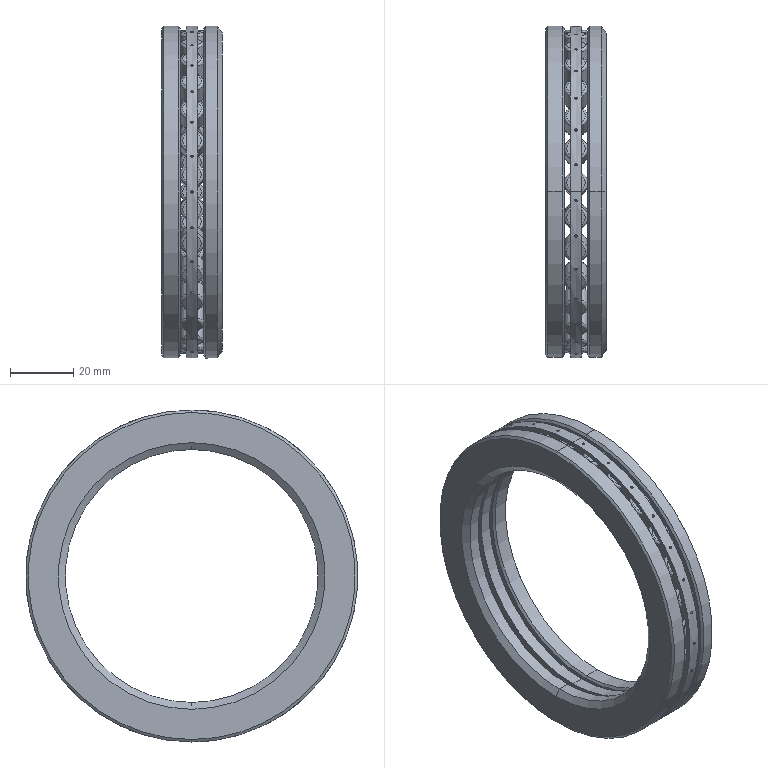Part | SolidWorks | features BaseBody 4 | 4 solids | 527 faces | box 19 x 105 x 105 mm | volume 55115 mm3 | cylinder 186 | torus 174 | plane 151 | cone 16 | commonest cylinder face diameters 7.5 x116 0.75 x58 105 x6 82 x4 80 x2